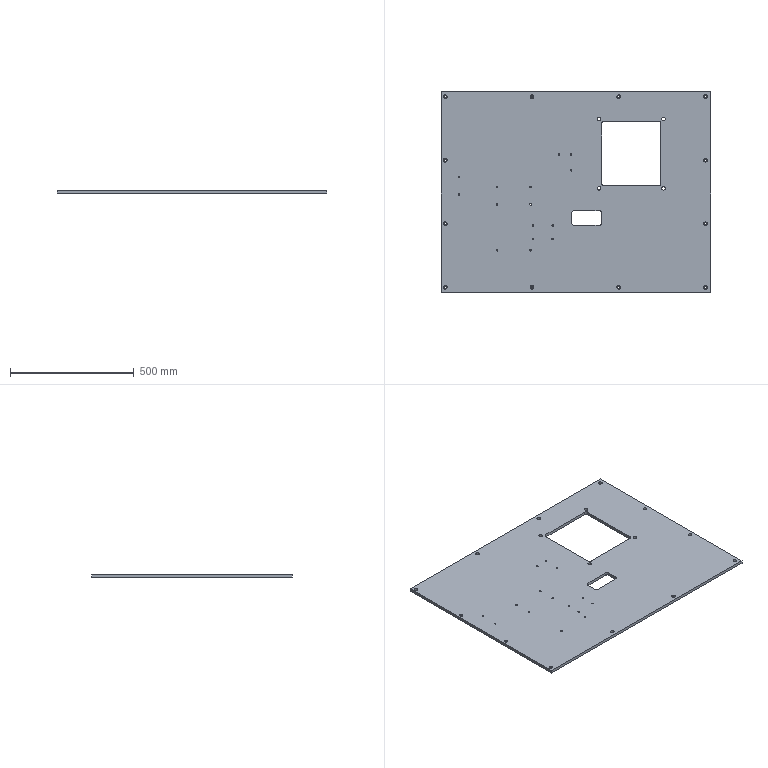Part | STEP file | X77-03002 | 1 solid | 120 faces | box 1087 x 810 x 12 mm | volume 9693894 mm3 | cylinder 94 | plane 26 | commonest cylinder face diameters 6.8 x30 9 x24 15 x24 14 x8 20 x8